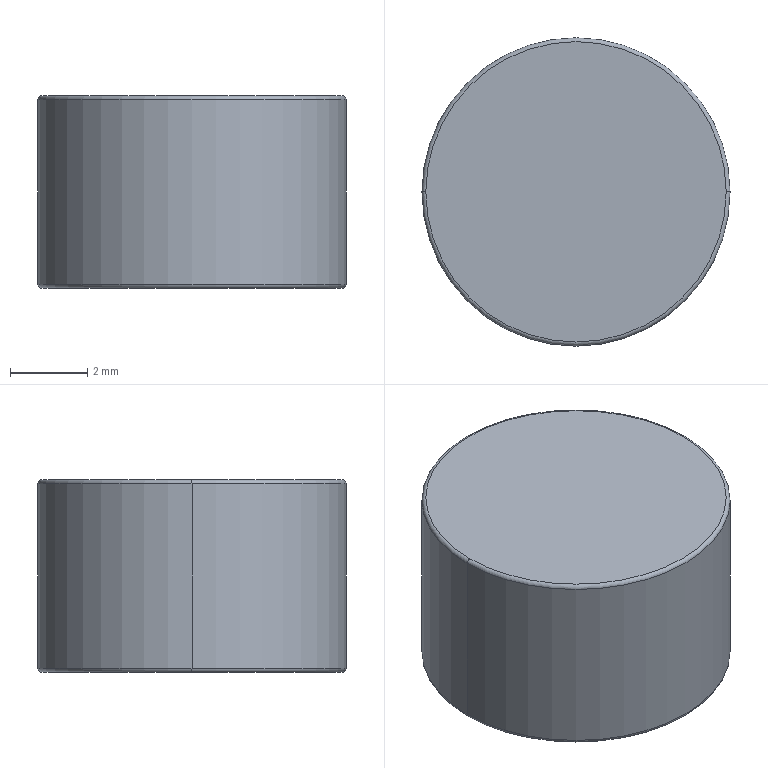Part | STEP file | HXN8-5 | 1 solid | 8 faces | box 8 x 8 x 5 mm | volume 251.22 mm3 | torus 4 | cylinder 2 | plane 2 | commonest cylinder face diameters 8 x2
STEP:
#1=CARTESIAN_POINT('',(0.,0.,0.));
#2=DIRECTION('',(0.,0.,1.));
#3=DIRECTION('',(1.,0.,0.));
#4=AXIS2_PLACEMENT_3D('',#1,#2,#3);
#5=CARTESIAN_POINT('',(-4.,0.,4.9));
#6=VERTEX_POINT('',#5);
#7=CARTESIAN_POINT('',(4.,0.,4.9));
#8=VERTEX_POINT('',#7);
#9=CARTESIAN_POINT('',(0.,0.,4.9));
#10=DIRECTION('',(0.,0.,-1.));
#11=DIRECTION('',(1.,0.,0.));
#12=AXIS2_PLACEMENT_3D('',#9,#10,#11);
#13=CIRCLE('',#12,4.);
#14=CARTESIAN_POINT('',(0.,0.,4.9));
#15=DIRECTION('',(0.,0.,1.));
#16=DIRECTION('',(1.,0.,0.));
#17=AXIS2_PLACEMENT_3D('',#14,#15,#16);
#18=TOROIDAL_SURFACE('',#17,3.9,0.1);
#19=CARTESIAN_POINT('',(6.283,0.));
#20=DIRECTION('',(-1.,0.));
#21=VECTOR('',#20,1.);
#22=LINE('',#19,#21);
#23=(GEOMETRIC_REPRESENTATION_CONTEXT(2)PARAMETRIC_REPRESENTATION_CONTEXT()REPRESENTATION_CONTEXT('',''));
#24=DEFINITIONAL_REPRESENTATION('',(#22),#23);
#25=PCURVE('',#18,#24);
#26=CARTESIAN_POINT('',(0.,0.,5.));
#27=DIRECTION('',(0.,0.,-1.));
#28=DIRECTION('',(-1.,0.,0.));
#29=AXIS2_PLACEMENT_3D('',#26,#27,#28);
#30=CYLINDRICAL_SURFACE('',#29,4.);
#31=CARTESIAN_POINT('',(-3.142,0.1));
#32=DIRECTION('',(1.,0.));
#33=VECTOR('',#32,1.);
#34=LINE('',#31,#33);
#35=(GEOMETRIC_REPRESENTATION_CONTEXT(2)PARAMETRIC_REPRESENTATION_CONTEXT()REPRESENTATION_CONTEXT('',''));
#36=DEFINITIONAL_REPRESENTATION('',(#34),#35);
#37=PCURVE('',#30,#36);
#38=SURFACE_CURVE('',#13,(#25,#37),.PCURVE_S1.);
#39=EDGE_CURVE('',#6,#8,#38,.T.);
#40=ORIENTED_EDGE('',*,*,#39,.F.);
#41=CARTESIAN_POINT('',(-3.9,0.,5.));
#42=VERTEX_POINT('',#41);
#43=CARTESIAN_POINT('',(-3.9,0.,4.9));
#44=DIRECTION('',(0.,1.,0.));
#45=DIRECTION('',(-1.,0.,0.));
#46=AXIS2_PLACEMENT_3D('',#43,#44,#45);
#47=CIRCLE('',#46,0.1);
#48=CARTESIAN_POINT('',(3.142,0.));
#49=DIRECTION('',(0.,1.));
#50=VECTOR('',#49,1.);
#51=LINE('',#48,#50);
#52=(GEOMETRIC_REPRESENTATION_CONTEXT(2)PARAMETRIC_REPRESENTATION_CONTEXT()REPRESENTATION_CONTEXT('',''));
#53=DEFINITIONAL_REPRESENTATION('',(#51),#52);
#54=PCURVE('',#18,#53);
#55=CARTESIAN_POINT('',(0.,0.,4.9));
#56=DIRECTION('',(0.,0.,1.));
#57=DIRECTION('',(1.,0.,0.));
#58=AXIS2_PLACEMENT_3D('',#55,#56,#57);
#59=TOROIDAL_SURFACE('',#58,3.9,0.1);
#60=CARTESIAN_POINT('',(3.142,0.));
#61=DIRECTION('',(0.,1.));
#62=VECTOR('',#61,1.);
#63=LINE('',#60,#62);
#64=(GEOMETRIC_REPRESENTATION_CONTEXT(2)PARAMETRIC_REPRESENTATION_CONTEXT()REPRESENTATION_CONTEXT('',''));
#65=DEFINITIONAL_REPRESENTATION('',(#63),#64);
#66=PCURVE('',#59,#65);
#67=SURFACE_CURVE('',#47,(#54,#66),.PCURVE_S1.);
#68=EDGE_CURVE('',#6,#42,#67,.T.);
#69=ORIENTED_EDGE('',*,*,#68,.T.);
#70=CARTESIAN_POINT('',(3.9,0.,5.));
#71=VERTEX_POINT('',#70);
#72=CARTESIAN_POINT('',(0.,0.,5.));
#73=DIRECTION('',(0.,0.,1.));
#74=DIRECTION('',(1.,0.,0.));
#75=AXIS2_PLACEMENT_3D('',#72,#73,#74);
#76=CIRCLE('',#75,3.9);
#77=CARTESIAN_POINT('',(0.,1.571));
#78=DIRECTION('',(1.,0.));
#79=VECTOR('',#78,1.);
#80=LINE('',#77,#79);
#81=(GEOMETRIC_REPRESENTATION_CONTEXT(2)PARAMETRIC_REPRESENTATION_CONTEXT()REPRESENTATION_CONTEXT('',''));
#82=DEFINITIONAL_REPRESENTATION('',(#80),#81);
#83=PCURVE('',#18,#82);
#84=CARTESIAN_POINT('',(0.,0.,5.));
#85=DIRECTION('',(0.,0.,1.));
#86=DIRECTION('',(1.,0.,0.));
#87=AXIS2_PLACEMENT_3D('',#84,#85,#86);
#88=PLANE('',#87);
#89=CARTESIAN_POINT('',(0.,0.));
#90=DIRECTION('',(1.,0.));
#91=AXIS2_PLACEMENT_2D('',#89,#90);
#92=CIRCLE('',#91,3.9);
#93=(GEOMETRIC_REPRESENTATION_CONTEXT(2)PARAMETRIC_REPRESENTATION_CONTEXT()REPRESENTATION_CONTEXT('',''));
#94=DEFINITIONAL_REPRESENTATION('',(#92),#93);
#95=PCURVE('',#88,#94);
#96=SURFACE_CURVE('',#76,(#83,#95),.PCURVE_S1.);
#97=EDGE_CURVE('',#71,#42,#96,.T.);
#98=ORIENTED_EDGE('',*,*,#97,.F.);
#99=CARTESIAN_POINT('',(3.9,0.,4.9));
#100=DIRECTION('',(0.,-1.,0.));
#101=DIRECTION('',(0.,0.,-1.));
#102=AXIS2_PLACEMENT_3D('',#99,#100,#101);
#103=CIRCLE('',#102,0.1);
#104=CARTESIAN_POINT('',(0.,-1.571));
#105=DIRECTION('',(0.,1.));
#106=VECTOR('',#105,1.);
#107=LINE('',#104,#106);
#108=(GEOMETRIC_REPRESENTATION_CONTEXT(2)PARAMETRIC_REPRESENTATION_CONTEXT()REPRESENTATION_CONTEXT('',''));
#109=DEFINITIONAL_REPRESENTATION('',(#107),#108);
#110=PCURVE('',#18,#109);
#111=CARTESIAN_POINT('',(6.283,-1.571));
#112=DIRECTION('',(0.,1.));
#113=VECTOR('',#112,1.);
#114=LINE('',#111,#113);
#115=(GEOMETRIC_REPRESENTATION_CONTEXT(2)PARAMETRIC_REPRESENTATION_CONTEXT()REPRESENTATION_CONTEXT('',''));
#116=DEFINITIONAL_REPRESENTATION('',(#114),#115);
#117=PCURVE('',#59,#116);
#118=SURFACE_CURVE('',#103,(#110,#117),.PCURVE_S1.);
#119=EDGE_CURVE('',#8,#71,#118,.T.);
#120=ORIENTED_EDGE('',*,*,#119,.F.);
#121=EDGE_LOOP('',(#40,#69,#98,#120));
#122=FACE_BOUND('',#121,.T.);
#123=ADVANCED_FACE('',(#122),#18,.T.);
#124=CARTESIAN_POINT('',(-3.9,0.,0.));
#125=VERTEX_POINT('',#124);
#126=CARTESIAN_POINT('',(3.9,0.,0.));
#127=VERTEX_POINT('',#126);
#128=CARTESIAN_POINT('',(0.,0.,0.));
#129=DIRECTION('',(0.,0.,-1.));
#130=DIRECTION('',(1.,0.,0.));
#131=AXIS2_PLACEMENT_3D('',#128,#129,#130);
#132=CIRCLE('',#131,3.9);
#133=CARTESIAN_POINT('',(0.,0.,0.1));
#134=DIRECTION('',(0.,0.,1.));
#135=DIRECTION('',(1.,0.,0.));
#136=AXIS2_PLACEMENT_3D('',#133,#134,#135);
#137=TOROIDAL_SURFACE('',#136,3.9,0.1);
#138=CARTESIAN_POINT('',(6.283,4.712));
#139=DIRECTION('',(-1.,0.));
#140=VECTOR('',#139,1.);
#141=LINE('',#138,#140);
#142=(GEOMETRIC_REPRESENTATION_CONTEXT(2)PARAMETRIC_REPRESENTATION_CONTEXT()REPRESENTATION_CONTEXT('',''));
#143=DEFINITIONAL_REPRESENTATION('',(#141),#142);
#144=PCURVE('',#137,#143);
#145=CARTESIAN_POINT('',(0.,0.,0.));
#146=DIRECTION('',(0.,0.,1.));
#147=DIRECTION('',(1.,0.,0.));
#148=AXIS2_PLACEMENT_3D('',#145,#146,#147);
#149=PLANE('',#148);
#150=CARTESIAN_POINT('',(3.9,0.));
#151=CARTESIAN_POINT('',(3.9,-6.755));
#152=CARTESIAN_POINT('',(-1.95,-3.377));
#153=CARTESIAN_POINT('',(-7.8,0.));
#154=CARTESIAN_POINT('',(-1.95,3.377));
#155=CARTESIAN_POINT('',(3.9,6.755));
#156=CARTESIAN_POINT('',(3.9,0.));
#157=(BOUNDED_CURVE()B_SPLINE_CURVE(2,(#150,#151,#152,#153,#154,#155,#156),.UNSPECIFIED.,.T.,.F.)B_SPLINE_CURVE_WITH_KNOTS((1,2,2,2,2,1),(-2.094,0.,2.094,4.189,6.283,8.378),.UNSPECIFIED.)CURVE()GEOMETRIC_REPRESENTATION_ITEM()RATIONAL_B_SPLINE_CURVE((1.,0.5,1.,0.5,1.,0.5,1.))REPRESENTATION_ITEM(''));
#158=(GEOMETRIC_REPRESENTATION_CONTEXT(2)PARAMETRIC_REPRESENTATION_CONTEXT()REPRESENTATION_CONTEXT('',''));
#159=DEFINITIONAL_REPRESENTATION('',(#157),#158);
#160=PCURVE('',#149,#159);
#161=SURFACE_CURVE('',#132,(#144,#160),.PCURVE_S1.);
#162=EDGE_CURVE('',#125,#127,#161,.T.);
#163=ORIENTED_EDGE('',*,*,#162,.F.);
#164=CARTESIAN_POINT('',(-4.,0.,0.1));
#165=VERTEX_POINT('',#164);
#166=CARTESIAN_POINT('',(-3.9,0.,0.1));
#167=DIRECTION('',(0.,1.,0.));
#168=DIRECTION('',(-1.,0.,0.));
#169=AXIS2_PLACEMENT_3D('',#166,#167,#168);
#170=CIRCLE('',#169,0.1);
#171=CARTESIAN_POINT('',(3.142,0.));
#172=DIRECTION('',(0.,1.));
#173=VECTOR('',#172,1.);
#174=LINE('',#171,#173);
#175=(GEOMETRIC_REPRESENTATION_CONTEXT(2)PARAMETRIC_REPRESENTATION_CONTEXT()REPRESENTATION_CONTEXT('',''));
#176=DEFINITIONAL_REPRESENTATION('',(#174),#175);
#177=PCURVE('',#137,#176);
#178=CARTESIAN_POINT('',(0.,0.,0.1));
#179=DIRECTION('',(0.,0.,1.));
#180=DIRECTION('',(1.,0.,0.));
#181=AXIS2_PLACEMENT_3D('',#178,#179,#180);
#182=TOROIDAL_SURFACE('',#181,3.9,0.1);
#183=CARTESIAN_POINT('',(3.142,0.));
#184=DIRECTION('',(0.,1.));
#185=VECTOR('',#184,1.);
#186=LINE('',#183,#185);
#187=(GEOMETRIC_REPRESENTATION_CONTEXT(2)PARAMETRIC_REPRESENTATION_CONTEXT()REPRESENTATION_CONTEXT('',''));
#188=DEFINITIONAL_REPRESENTATION('',(#186),#187);
#189=PCURVE('',#182,#188);
#190=SURFACE_CURVE('',#170,(#177,#189),.PCURVE_S1.);
#191=EDGE_CURVE('',#125,#165,#190,.T.);
#192=ORIENTED_EDGE('',*,*,#191,.T.);
#193=CARTESIAN_POINT('',(4.,0.,0.1));
#194=VERTEX_POINT('',#193);
#195=CARTESIAN_POINT('',(0.,0.,0.1));
#196=DIRECTION('',(0.,0.,1.));
#197=DIRECTION('',(1.,0.,0.));
#198=AXIS2_PLACEMENT_3D('',#195,#196,#197);
#199=CIRCLE('',#198,4.);
#200=CARTESIAN_POINT('',(0.,6.283));
#201=DIRECTION('',(1.,0.));
#202=VECTOR('',#201,1.);
#203=LINE('',#200,#202);
#204=(GEOMETRIC_REPRESENTATION_CONTEXT(2)PARAMETRIC_REPRESENTATION_CONTEXT()REPRESENTATION_CONTEXT('',''));
#205=DEFINITIONAL_REPRESENTATION('',(#203),#204);
#206=PCURVE('',#137,#205);
#207=CARTESIAN_POINT('',(3.142,4.9));
#208=DIRECTION('',(-1.,0.));
#209=VECTOR('',#208,1.);
#210=LINE('',#207,#209);
#211=(GEOMETRIC_REPRESENTATION_CONTEXT(2)PARAMETRIC_REPRESENTATION_CONTEXT()REPRESENTATION_CONTEXT('',''));
#212=DEFINITIONAL_REPRESENTATION('',(#210),#211);
#213=PCURVE('',#30,#212);
#214=SURFACE_CURVE('',#199,(#206,#213),.PCURVE_S1.);
#215=EDGE_CURVE('',#194,#165,#214,.T.);
#216=ORIENTED_EDGE('',*,*,#215,.F.);
#217=CARTESIAN_POINT('',(3.9,0.,0.1));
#218=DIRECTION('',(0.,-1.,0.));
#219=DIRECTION('',(0.,0.,-1.));
#220=AXIS2_PLACEMENT_3D('',#217,#218,#219);
#221=CIRCLE('',#220,0.1);
#222=CARTESIAN_POINT('',(0.,4.712));
#223=DIRECTION('',(0.,1.));
#224=VECTOR('',#223,1.);
#225=LINE('',#222,#224);
#226=(GEOMETRIC_REPRESENTATION_CONTEXT(2)PARAMETRIC_REPRESENTATION_CONTEXT()REPRESENTATION_CONTEXT('',''));
#227=DEFINITIONAL_REPRESENTATION('',(#225),#226);
#228=PCURVE('',#137,#227);
#229=CARTESIAN_POINT('',(6.283,4.712));
#230=DIRECTION('',(0.,1.));
#231=VECTOR('',#230,1.);
#232=LINE('',#229,#231);
#233=(GEOMETRIC_REPRESENTATION_CONTEXT(2)PARAMETRIC_REPRESENTATION_CONTEXT()REPRESENTATION_CONTEXT('',''));
#234=DEFINITIONAL_REPRESENTATION('',(#232),#233);
#235=PCURVE('',#182,#234);
#236=SURFACE_CURVE('',#221,(#228,#235),.PCURVE_S1.);
#237=EDGE_CURVE('',#127,#194,#236,.T.);
#238=ORIENTED_EDGE('',*,*,#237,.F.);
#239=EDGE_LOOP('',(#163,#192,#216,#238));
#240=FACE_BOUND('',#239,.T.);
#241=ADVANCED_FACE('',(#240),#137,.T.);
#242=ORIENTED_EDGE('',*,*,#39,.T.);
#243=CARTESIAN_POINT('',(4.,0.,5.));
#244=DIRECTION('',(0.,0.,-1.));
#245=VECTOR('',#244,1.);
#246=LINE('',#243,#245);
#247=CARTESIAN_POINT('',(3.142,0.));
#248=DIRECTION('',(0.,1.));
#249=VECTOR('',#248,1.);
#250=LINE('',#247,#249);
#251=(GEOMETRIC_REPRESENTATION_CONTEXT(2)PARAMETRIC_REPRESENTATION_CONTEXT()REPRESENTATION_CONTEXT('',''));
#252=DEFINITIONAL_REPRESENTATION('',(#250),#251);
#253=PCURVE('',#30,#252);
#254=CARTESIAN_POINT('',(0.,0.,5.));
#255=DIRECTION('',(0.,0.,-1.));
#256=DIRECTION('',(-1.,0.,0.));
#257=AXIS2_PLACEMENT_3D('',#254,#255,#256);
#258=CYLINDRICAL_SURFACE('',#257,4.);
#259=CARTESIAN_POINT('',(3.142,0.));
#260=DIRECTION('',(0.,1.));
#261=VECTOR('',#260,1.);
#262=LINE('',#259,#261);
#263=(GEOMETRIC_REPRESENTATION_CONTEXT(2)PARAMETRIC_REPRESENTATION_CONTEXT()REPRESENTATION_CONTEXT('',''));
#264=DEFINITIONAL_REPRESENTATION('',(#262),#263);
#265=PCURVE('',#258,#264);
#266=SURFACE_CURVE('',#246,(#253,#265),.PCURVE_S1.);
#267=EDGE_CURVE('',#8,#194,#266,.T.);
#268=ORIENTED_EDGE('',*,*,#267,.T.);
#269=ORIENTED_EDGE('',*,*,#215,.T.);
#270=CARTESIAN_POINT('',(-4.,0.,5.));
#271=DIRECTION('',(0.,0.,-1.));
#272=VECTOR('',#271,1.);
#273=LINE('',#270,#272);
#274=CARTESIAN_POINT('',(0.,0.));
#275=DIRECTION('',(0.,1.));
#276=VECTOR('',#275,1.);
#277=LINE('',#274,#276);
#278=(GEOMETRIC_REPRESENTATION_CONTEXT(2)PARAMETRIC_REPRESENTATION_CONTEXT()REPRESENTATION_CONTEXT('',''));
#279=DEFINITIONAL_REPRESENTATION('',(#277),#278);
#280=PCURVE('',#30,#279);
#281=CARTESIAN_POINT('',(6.283,0.));
#282=DIRECTION('',(0.,1.));
#283=VECTOR('',#282,1.);
#284=LINE('',#281,#283);
#285=(GEOMETRIC_REPRESENTATION_CONTEXT(2)PARAMETRIC_REPRESENTATION_CONTEXT()REPRESENTATION_CONTEXT('',''));
#286=DEFINITIONAL_REPRESENTATION('',(#284),#285);
#287=PCURVE('',#258,#286);
#288=SURFACE_CURVE('',#273,(#280,#287),.PCURVE_S1.);
#289=EDGE_CURVE('',#6,#165,#288,.T.);
#290=ORIENTED_EDGE('',*,*,#289,.F.);
#291=EDGE_LOOP('',(#242,#268,#269,#290));
#292=FACE_BOUND('',#291,.T.);
#293=ADVANCED_FACE('',(#292),#30,.T.);
#294=ORIENTED_EDGE('',*,*,#267,.F.);
#295=CARTESIAN_POINT('',(0.,0.,4.9));
#296=DIRECTION('',(0.,0.,-1.));
#297=DIRECTION('',(1.,0.,0.));
#298=AXIS2_PLACEMENT_3D('',#295,#296,#297);
#299=CIRCLE('',#298,4.);
#300=CARTESIAN_POINT('',(3.142,0.1));
#301=DIRECTION('',(1.,0.));
#302=VECTOR('',#301,1.);
#303=LINE('',#300,#302);
#304=(GEOMETRIC_REPRESENTATION_CONTEXT(2)PARAMETRIC_REPRESENTATION_CONTEXT()REPRESENTATION_CONTEXT('',''));
#305=DEFINITIONAL_REPRESENTATION('',(#303),#304);
#306=PCURVE('',#258,#305);
#307=CARTESIAN_POINT('',(6.283,0.));
#308=DIRECTION('',(-1.,0.));
#309=VECTOR('',#308,1.);
#310=LINE('',#307,#309);
#311=(GEOMETRIC_REPRESENTATION_CONTEXT(2)PARAMETRIC_REPRESENTATION_CONTEXT()REPRESENTATION_CONTEXT('',''));
#312=DEFINITIONAL_REPRESENTATION('',(#310),#311);
#313=PCURVE('',#59,#312);
#314=SURFACE_CURVE('',#299,(#306,#313),.PCURVE_S1.);
#315=EDGE_CURVE('',#8,#6,#314,.T.);
#316=ORIENTED_EDGE('',*,*,#315,.T.);
#317=ORIENTED_EDGE('',*,*,#289,.T.);
#318=CARTESIAN_POINT('',(0.,0.,0.1));
#319=DIRECTION('',(0.,0.,1.));
#320=DIRECTION('',(1.,0.,0.));
#321=AXIS2_PLACEMENT_3D('',#318,#319,#320);
#322=CIRCLE('',#321,4.);
#323=CARTESIAN_POINT('',(9.425,4.9));
#324=DIRECTION('',(-1.,0.));
#325=VECTOR('',#324,1.);
#326=LINE('',#323,#325);
#327=(GEOMETRIC_REPRESENTATION_CONTEXT(2)PARAMETRIC_REPRESENTATION_CONTEXT()REPRESENTATION_CONTEXT('',''));
#328=DEFINITIONAL_REPRESENTATION('',(#326),#327);
#329=PCURVE('',#258,#328);
#330=CARTESIAN_POINT('',(0.,6.283));
#331=DIRECTION('',(1.,0.));
#332=VECTOR('',#331,1.);
#333=LINE('',#330,#332);
#334=(GEOMETRIC_REPRESENTATION_CONTEXT(2)PARAMETRIC_REPRESENTATION_CONTEXT()REPRESENTATION_CONTEXT('',''));
#335=DEFINITIONAL_REPRESENTATION('',(#333),#334);
#336=PCURVE('',#182,#335);
#337=SURFACE_CURVE('',#322,(#329,#336),.PCURVE_S1.);
#338=EDGE_CURVE('',#165,#194,#337,.T.);
#339=ORIENTED_EDGE('',*,*,#338,.T.);
#340=EDGE_LOOP('',(#294,#316,#317,#339));
#341=FACE_BOUND('',#340,.T.);
#342=ADVANCED_FACE('',(#341),#258,.T.);
#343=ORIENTED_EDGE('',*,*,#97,.T.);
#344=CARTESIAN_POINT('',(0.,0.,5.));
#345=DIRECTION('',(0.,0.,1.));
#346=DIRECTION('',(1.,0.,0.));
#347=AXIS2_PLACEMENT_3D('',#344,#345,#346);
#348=CIRCLE('',#347,3.9);
#349=CARTESIAN_POINT('',(0.,0.));
#350=DIRECTION('',(1.,0.));
#351=AXIS2_PLACEMENT_2D('',#349,#350);
#352=CIRCLE('',#351,3.9);
#353=(GEOMETRIC_REPRESENTATION_CONTEXT(2)PARAMETRIC_REPRESENTATION_CONTEXT()REPRESENTATION_CONTEXT('',''));
#354=DEFINITIONAL_REPRESENTATION('',(#352),#353);
#355=PCURVE('',#88,#354);
#356=CARTESIAN_POINT('',(0.,1.571));
#357=DIRECTION('',(1.,0.));
#358=VECTOR('',#357,1.);
#359=LINE('',#356,#358);
#360=(GEOMETRIC_REPRESENTATION_CONTEXT(2)PARAMETRIC_REPRESENTATION_CONTEXT()REPRESENTATION_CONTEXT('',''));
#361=DEFINITIONAL_REPRESENTATION('',(#359),#360);
#362=PCURVE('',#59,#361);
#363=SURFACE_CURVE('',#348,(#355,#362),.PCURVE_S1.);
#364=EDGE_CURVE('',#42,#71,#363,.T.);
#365=ORIENTED_EDGE('',*,*,#364,.T.);
#366=EDGE_LOOP('',(#343,#365));
#367=FACE_BOUND('',#366,.T.);
#368=ADVANCED_FACE('',(#367),#88,.T.);
#369=CARTESIAN_POINT('',(0.,0.,0.));
#370=DIRECTION('',(0.,0.,-1.));
#371=DIRECTION('',(1.,0.,0.));
#372=AXIS2_PLACEMENT_3D('',#369,#370,#371);
#373=CIRCLE('',#372,3.9);
#374=CARTESIAN_POINT('',(3.9,0.));
#375=CARTESIAN_POINT('',(3.9,-6.755));
#376=CARTESIAN_POINT('',(-1.95,-3.377));
#377=CARTESIAN_POINT('',(-7.8,0.));
#378=CARTESIAN_POINT('',(-1.95,3.377));
#379=CARTESIAN_POINT('',(3.9,6.755));
#380=CARTESIAN_POINT('',(3.9,0.));
#381=(BOUNDED_CURVE()B_SPLINE_CURVE(2,(#374,#375,#376,#377,#378,#379,#380),.UNSPECIFIED.,.T.,.F.)B_SPLINE_CURVE_WITH_KNOTS((1,2,2,2,2,1),(-2.094,0.,2.094,4.189,6.283,8.378),.UNSPECIFIED.)CURVE()GEOMETRIC_REPRESENTATION_ITEM()RATIONAL_B_SPLINE_CURVE((1.,0.5,1.,0.5,1.,0.5,1.))REPRESENTATION_ITEM(''));
#382=(GEOMETRIC_REPRESENTATION_CONTEXT(2)PARAMETRIC_REPRESENTATION_CONTEXT()REPRESENTATION_CONTEXT('',''));
#383=DEFINITIONAL_REPRESENTATION('',(#381),#382);
#384=PCURVE('',#149,#383);
#385=CARTESIAN_POINT('',(6.283,4.712));
#386=DIRECTION('',(-1.,0.));
#387=VECTOR('',#386,1.);
#388=LINE('',#385,#387);
#389=(GEOMETRIC_REPRESENTATION_CONTEXT(2)PARAMETRIC_REPRESENTATION_CONTEXT()REPRESENTATION_CONTEXT('',''));
#390=DEFINITIONAL_REPRESENTATION('',(#388),#389);
#391=PCURVE('',#182,#390);
#392=SURFACE_CURVE('',#373,(#384,#391),.PCURVE_S1.);
#393=EDGE_CURVE('',#127,#125,#392,.T.);
#394=ORIENTED_EDGE('',*,*,#393,.T.);
#395=ORIENTED_EDGE('',*,*,#162,.T.);
#396=EDGE_LOOP('',(#394,#395));
#397=FACE_BOUND('',#396,.T.);
#398=ADVANCED_FACE('',(#397),#149,.F.);
#399=ORIENTED_EDGE('',*,*,#191,.F.);
#400=ORIENTED_EDGE('',*,*,#393,.F.);
#401=ORIENTED_EDGE('',*,*,#237,.T.);
#402=ORIENTED_EDGE('',*,*,#338,.F.);
#403=EDGE_LOOP('',(#399,#400,#401,#402));
#404=FACE_BOUND('',#403,.T.);
#405=ADVANCED_FACE('',(#404),#182,.T.);
#406=ORIENTED_EDGE('',*,*,#68,.F.);
#407=ORIENTED_EDGE('',*,*,#315,.F.);
#408=ORIENTED_EDGE('',*,*,#119,.T.);
#409=ORIENTED_EDGE('',*,*,#364,.F.);
#410=EDGE_LOOP('',(#406,#407,#408,#409));
#411=FACE_BOUND('',#410,.T.);
#412=ADVANCED_FACE('',(#411),#59,.T.);
#413=CLOSED_SHELL('',(#123,#241,#293,#342,#368,#398,#405,#412));
#414=MANIFOLD_SOLID_BREP('',#413);
#415=(LENGTH_UNIT()NAMED_UNIT(*)SI_UNIT(.MILLI.,.METRE.));
#416=UNCERTAINTY_MEASURE_WITH_UNIT(LENGTH_MEASURE(0.0000001),#415,'','');
#417=(NAMED_UNIT(*)PLANE_ANGLE_UNIT()SI_UNIT($,.RADIAN.));
#418=(NAMED_UNIT(*)SI_UNIT($,.STERADIAN.)SOLID_ANGLE_UNIT());
#419=(GEOMETRIC_REPRESENTATION_CONTEXT(3)GLOBAL_UNCERTAINTY_ASSIGNED_CONTEXT((#416))GLOBAL_UNIT_ASSIGNED_CONTEXT((#415,#417,#418))REPRESENTATION_CONTEXT('',''));
#420=ADVANCED_BREP_SHAPE_REPRESENTATION('',(#4,#414),#419);